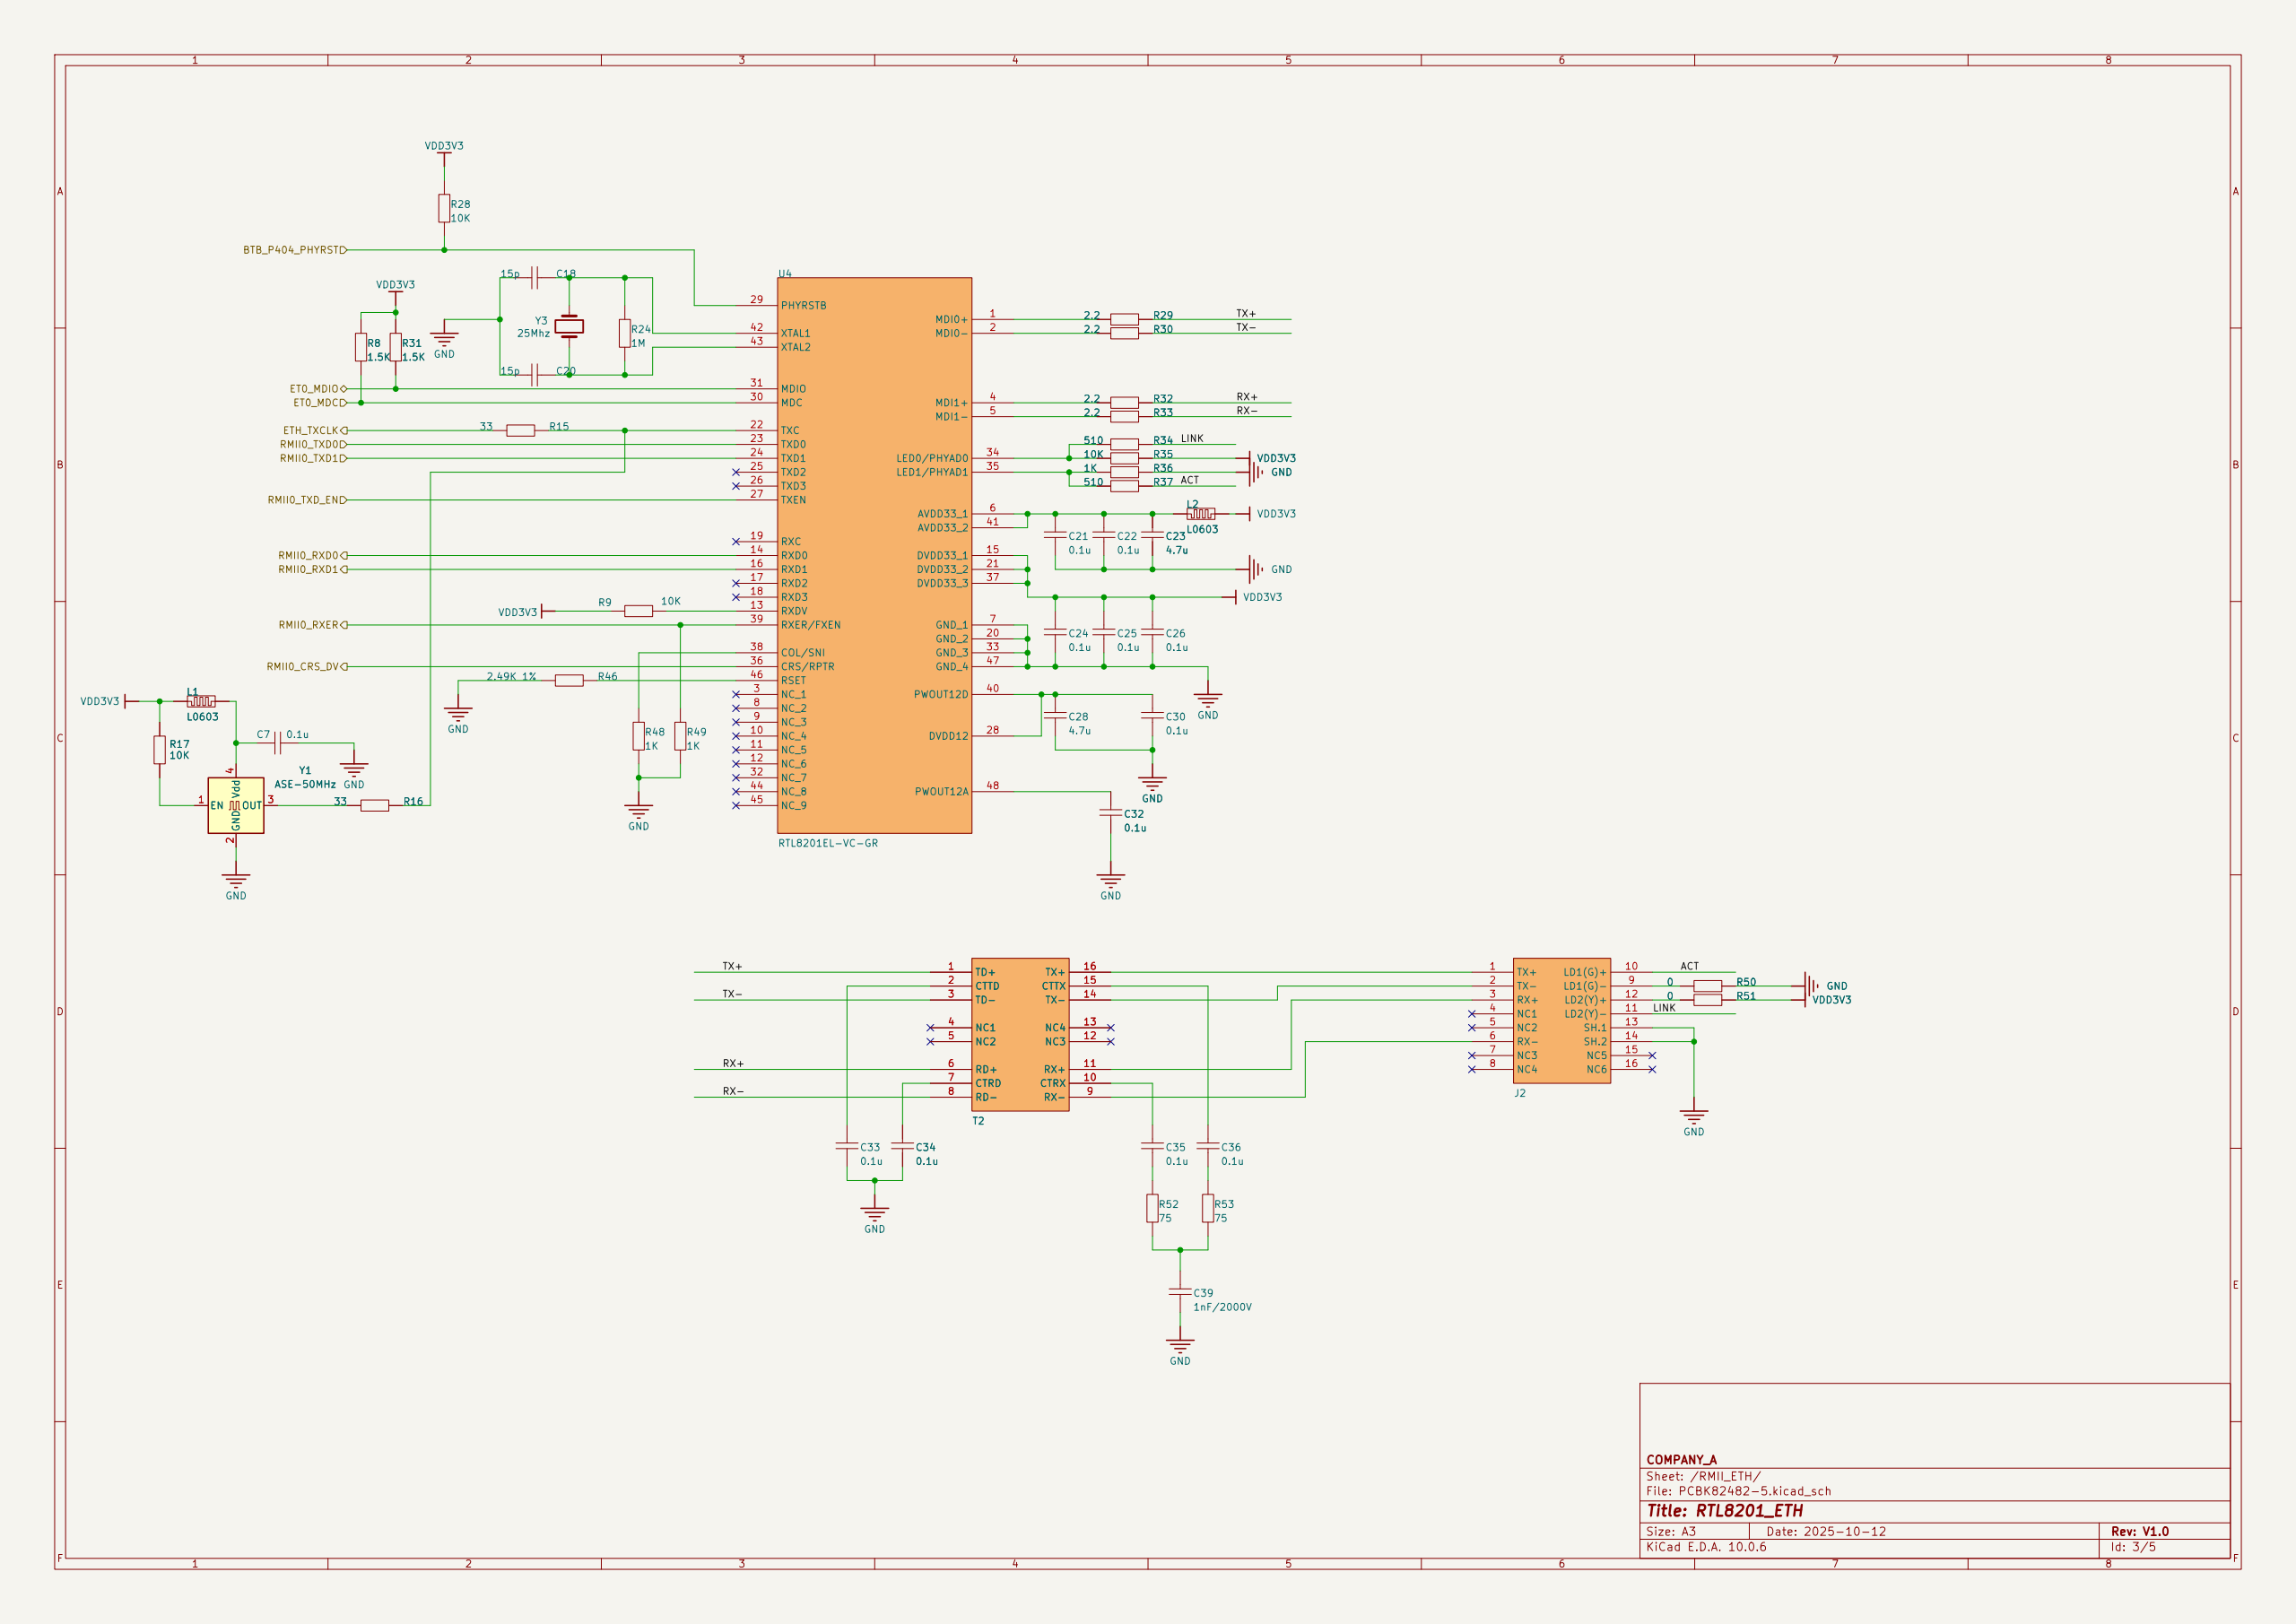Circuit board | KiCad | 154 parts | 201 nets | one sheet of the schematic
Parts on this sheet (reference | value | footprint):
C18 | 15p | Library:C0603
C20 | 15p | Library:C0603
C21 | 0.1u | Library:C0603
C22 | 0.1u | Library:C0603
C23 | 4.7u | Library:C1206
C24
C25
C26
C28 | 4.7u | Library:C0603
C32
C33
C34
C35
C36
C39 | 1nF/2000V | Library:C1808
C7
J2 | RJ45 | Library:RJ45_1X1L_20U
L1
L2
R15 | 33 | Library:R0603
R16 | 33 | Library:R0603
R17 | 10K | Library:R0603
R24 | 1M | Library:R0603
R28 | 10K | Library:R0603
R29 | 2.2 | Library:R0603
R30 | 2.2 | Library:R0603
R31 | 1.5K | Library:R0603
R32 | 2.2 | Library:R0603
R33 | 2.2 | Library:R0603
R34 | 510 | Library:R0603
R35 | 10K | Library:R0603
R36 | 1K | Library:R0603
R37 | 510 | Library:R0603
R46 | 2.49K 1% | Library:R0603
R48 | 1K | Library:R0603
R49 | 1K | Library:R0603
R50 | 0 | Library:R0603
R51 | 0 | Library:R0603
R52 | 75 | Library:R0805
R53 | 75 | Library:R0805
R8 | 1.5K | Library:R0603
R9 | 10K | Library:R0603
T2 | TS6121C | Library:TS6121C
Y1 | ASE-50MHz | Oscillator:Oscillator_SMD_Abracon_ASE-4Pin_3.2x2.5mm
Y3 | 25Mhz | Crystal:Crystal_SMD_5032-2Pin_5.0x3.2mm_HandSoldering
Nets of these parts (net: part-pin ...):
/RMII_ETH/ACT: J2-10 R37-2
/RMII_ETH/LINK: J2-11 R34-2
/RMII_ETH/RX+: R32-2 T2-6
/RMII_ETH/RX-: R33-2 T2-8
/RMII_ETH/TX+: R29-2 T2-1
/RMII_ETH/TX-: R30-2 T2-3
/Vision_Interface/BTB_P404_PHYRST: R28-1
/Vision_Interface/ET0_MDC: R8-1
/Vision_Interface/ET0_MDIO: R31-1
/Vision_Interface/REF50CK0: R15-1
/Vision_Interface/RMII0_RX_ER: R49-2
GND: C7-1 C18-2 C20-2 C21-1 C22-1 C23-1 C24-1 C25-1 C26-1 C28-1 C32-1 C33-1 C34-1 C39-1 J2-13 J2-14 R36-2 R46-1 R48-1 R49-1 R50-2 Y1-2
Net-(C35-Pad1): C35-1 R52-2
Net-(C36-Pad1): C36-1 R53-2
Net-(C39-Pad2): C39-2 R52-1 R53-1
Net-(J2-LD1(G)-): J2-9 R50-1
Net-(J2-LD2(Y)+): J2-12 R51-1
Net-(J2-RX+): J2-3 T2-11
Net-(J2-RX-): J2-6 T2-9
Net-(J2-TX+): J2-1 T2-16
Net-(J2-TX-): J2-2 T2-14
Net-(T2-CTRD): C34-2 T2-7
Net-(T2-CTRX): C35-2 T2-10
Net-(T2-CTTD): C33-2 T2-2
Net-(T2-CTTX): C36-2 T2-15
Net-(U4-AVDD33_1): C21-2 C22-2 C23-2 L2-1
Net-(U4-COL{slash}SNI): R48-2
Net-(U4-DVDD12): C28-2
Net-(U4-LED0{slash}PHYAD0): R34-1 R35-1
Net-(U4-LED1{slash}PHYAD1): R36-1 R37-1
Net-(U4-MDI0+): R29-1
Net-(U4-MDI0-): R30-1
Net-(U4-MDI1+): R32-1
Net-(U4-MDI1-): R33-1
Net-(U4-PWOUT12A): C32-2
Net-(U4-RSET): R46-2
Net-(U4-RXDV): R9-1
Net-(U4-TXC): R15-2 R16-2
Net-(U4-XTAL1): C18-1 R24-1 Y3-2
Net-(U4-XTAL2): C20-1 R24-2 Y3-1
Net-(Y1-EN): R17-2 Y1-1
Net-(Y1-OUT): R16-1 Y1-3
Net-(Y1-Vdd): C7-2 L1-2 Y1-4
VDD3V3: C24-2 C25-2 C26-2 L1-1 L2-2 R8-2 R9-2 R17-1 R28-2 R31-2 R35-2 R51-2
unconnected-(J2-NC1-Pad4): J2-4
unconnected-(J2-NC2-Pad5): J2-5
unconnected-(J2-NC3-Pad7): J2-7
unconnected-(J2-NC4-Pad8): J2-8
unconnected-(J2-NC5-Pad15): J2-15
unconnected-(J2-NC6-Pad16): J2-16
unconnected-(T2-NC1-Pad4): T2-4
unconnected-(T2-NC2-Pad5): T2-5
unconnected-(T2-NC3-Pad12): T2-12
unconnected-(T2-NC4-Pad13): T2-13